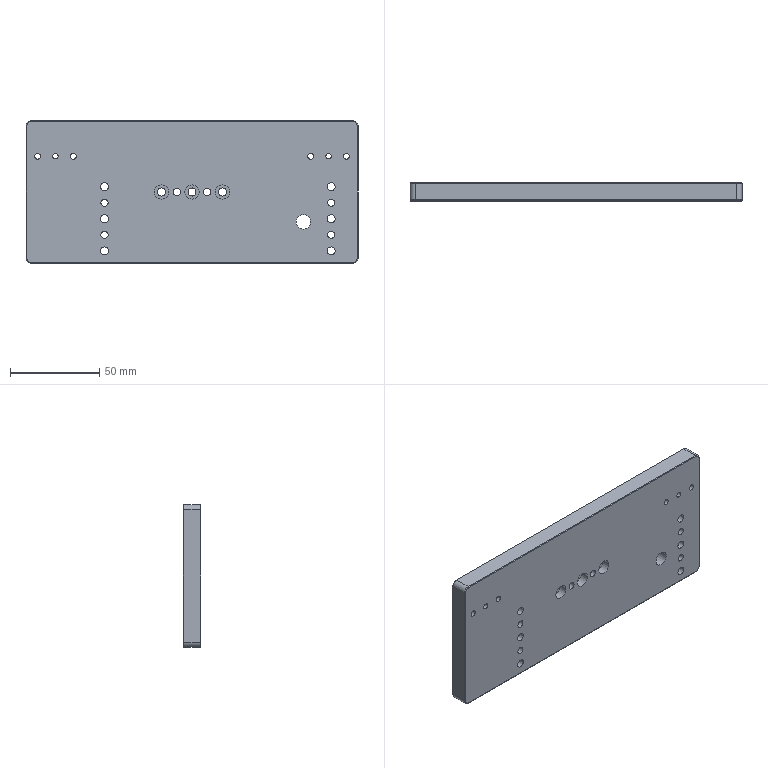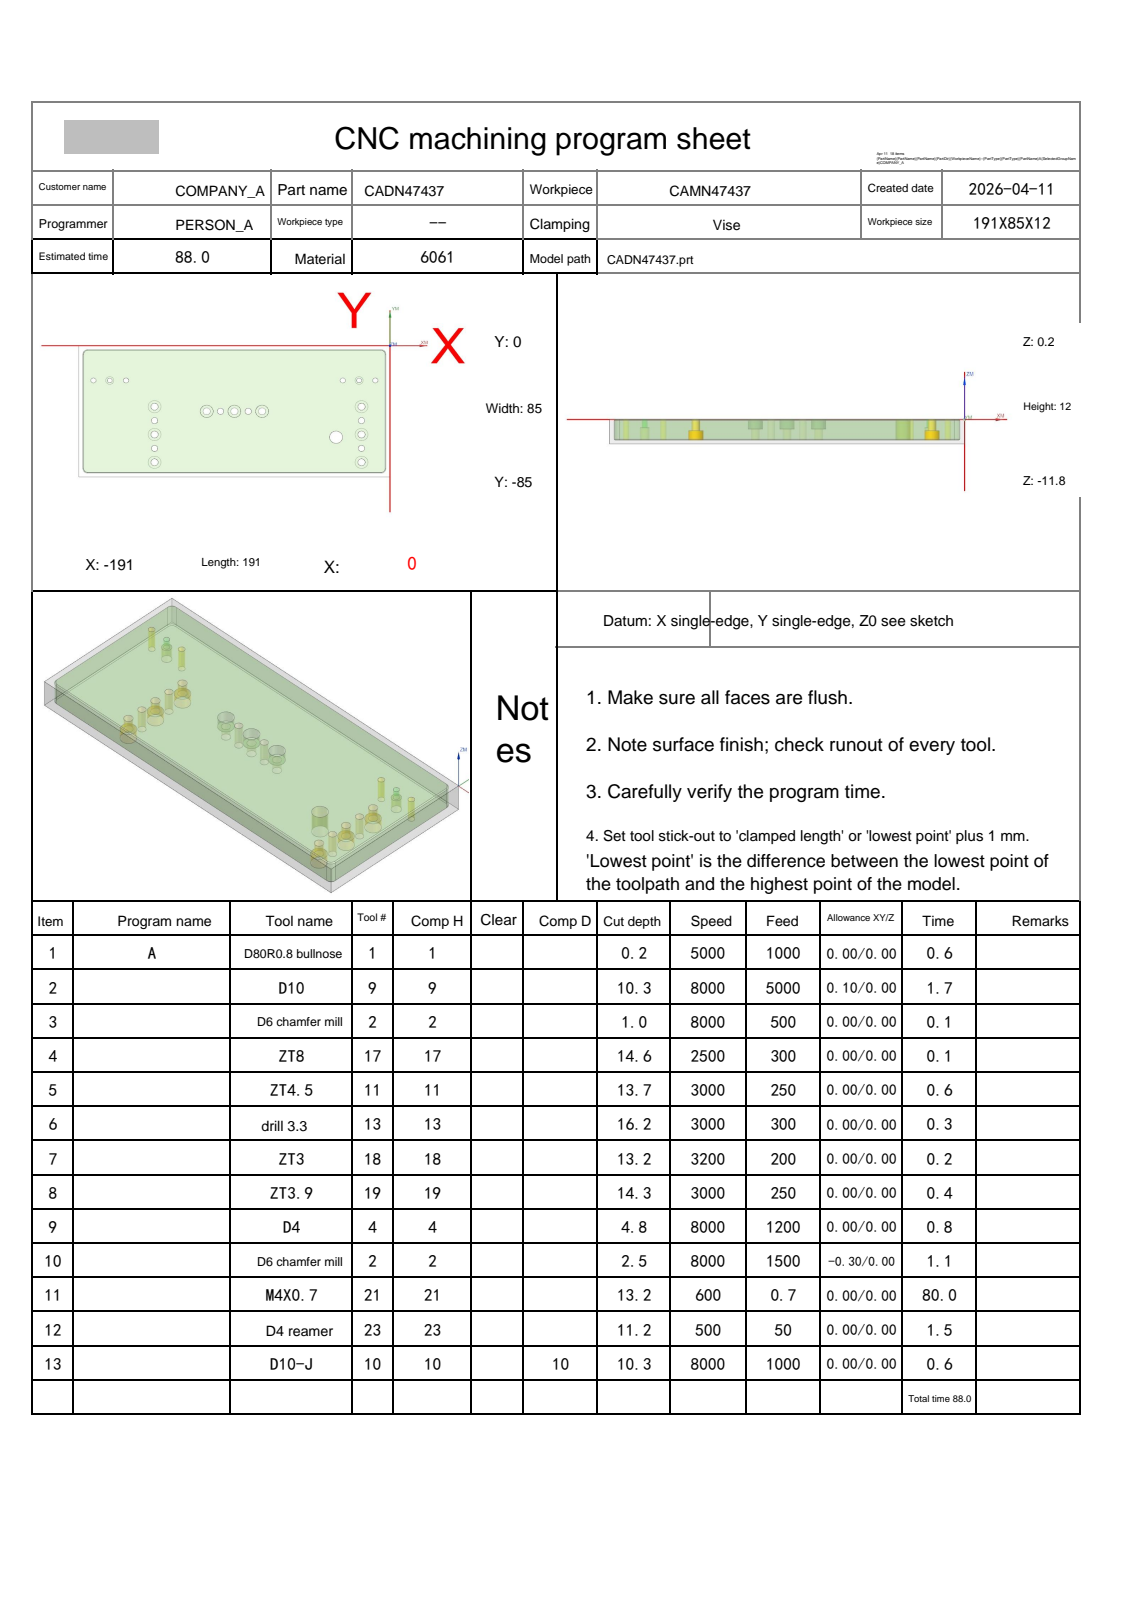NC program | NX | posted by the shop | part box 186 x 10 x 80 mm
Whole program:
%
O0001
(Machine time: 164.60 MIN)
(===Total Tool:12===)
(T1=D80R0.8 bullnose D=80.  R=0.8  D-  H01 Z=-0.   )
(T9=D10     D=10.  R=0.   D-  H09 Z=-10.1 )
(T2=D6 chamfer mill   D=6.   R=0.   D-  H02 Z=-2.3  )
(T17=ZT8    D=8.   DR_a=118 D-  H17 Z=-14.4 )
(T11=ZT4.5  D=4.5  DR_a=118 D-  H11 Z=-13.5 )
(T13=drill 3.3  D=3.3  DR_a=118 D-  H13 Z=-15.99)
(T18=ZT3    D=3.   DR_a=118 D-  H18 Z=-13.  )
(T19=ZT3.9  D=3.9  DR_a=120 D-  H19 Z=-14.13)
(T4=D4      D=4.   R=0.   D4  H04 Z=-4.6  )
(T21=M4X0.7 D=3.3  DR_a=180 D-  H21 Z=-13.  )
(T23=D4 reamer   D=4.   DR_a=180 D-  H23 Z=-11.  )
(T10=D10-J  D=10.  R=0.   D10 H10 Z=-10.1 )
G80 G90 G17 G49 G40
G91 G28 Z0
M01
N1 T01 M06
(D80R0.8 bullnose  D=80. R=0.8 H=01 ce=0.00 di=0.00)
G00 G90 G54 X42.5 Y-69.167 M03 S5000
G43 H01 Z20.
M08
Z2.
G01 Z0.0 F1000.
X37.5
X-228.5
Y-15.833
X37.5
X42.5
Z2.
G00 Z20.
G91 G28 Z0.0
M05
M09
G91 G28 Z0.0
M01
N2 T09 M06
(D10  D=10. R=0. H=09 ce=0.10 di=0.00)
G00 G90 G54 X-95.5 Y2.6 M03 S8000
G43 H09 Z20.
M08
Z.5
G01 X-5.5 Z.378 F5000.
G02 X2.6 Y-5.5 Z.361 I0.0 J-8.1
G01 Y-79.5 Z.261
G02 X-5.5 Y-87.6 Z.243 I-8.1 J0.0
G01 X-185.5 Z0.0
G02 X-193.6 Y-79.5 Z-.018 I0.0 J8.1
G01 Y-5.5 Z-.118
G02 X-185.5 Y2.6 Z-.135 I8.1 J0.0
G01 X-5.5 Z-.379
G02 X2.6 Y-5.5 Z-.396 I0.0 J-8.1
G01 Y-79.5 Z-.497
G02 X-5.5 Y-87.6 Z-.514 I-8.1 J0.0
G01 X-185.5 Z-.758
G02 X-193.6 Y-79.5 Z-.775 I0.0 J8.1
G01 Y-5.5 Z-.875
G02 X-185.5 Y2.6 Z-.892 I8.1 J0.0
G01 X-5.5 Z-1.136
G02 X2.6 Y-5.5 Z-1.153 I0.0 J-8.1
G01 Y-79.5 Z-1.254
G02 X-5.5 Y-87.6 Z-1.271 I-8.1 J0.0
G01 X-185.5 Z-1.515
G02 X-193.6 Y-79.5 Z-1.532 I0.0 J8.1
G01 Y-5.5 Z-1.632
G02 X-185.5 Y2.6 Z-1.65 I8.1 J0.0
G01 X-5.5 Z-1.893
G02 X2.6 Y-5.5 Z-1.911 I0.0 J-8.1
G01 Y-79.5 Z-2.011
G02 X-5.5 Y-87.6 Z-2.028 I-8.1 J0.0
G01 X-185.5 Z-2.272
G02 X-193.6 Y-79.5 Z-2.289 I0.0 J8.1
G01 Y-5.5 Z-2.389
G02 X-185.5 Y2.6 Z-2.407 I8.1 J0.0
G01 X-5.5 Z-2.65
G02 X2.6 Y-5.5 Z-2.668 I0.0 J-8.1
G01 Y-79.5 Z-2.768
G02 X-5.5 Y-87.6 Z-2.785 I-8.1 J0.0
G01 X-185.5 Z-3.029
G02 X-193.6 Y-79.5 Z-3.046 I0.0 J8.1
G01 Y-5.5 Z-3.147
G02 X-185.5 Y2.6 Z-3.164 I8.1 J0.0
G01 X-5.5 Z-3.408
G02 X2.6 Y-5.5 Z-3.425 I0.0 J-8.1
G01 Y-79.5 Z-3.525
G02 X-5.5 Y-87.6 Z-3.542 I-8.1 J0.0
G01 X-185.5 Z-3.786
G02 X-193.6 Y-79.5 Z-3.803 I0.0 J8.1
G01 Y-5.5 Z-3.904
G02 X-185.5 Y2.6 Z-3.921 I8.1 J0.0
G01 X-5.5 Z-4.165
G02 X2.6 Y-5.5 Z-4.182 I0.0 J-8.1
G01 Y-79.5 Z-4.282
G02 X-5.5 Y-87.6 Z-4.3 I-8.1 J0.0
G01 X-185.5 Z-4.543
G02 X-193.6 Y-79.5 Z-4.561 I0.0 J8.1
G01 Y-5.5 Z-4.661
G02 X-185.5 Y2.6 Z-4.678 I8.1 J0.0
G01 X-5.5 Z-4.922
G02 X2.6 Y-5.5 Z-4.939 I0.0 J-8.1
G01 Y-79.5 Z-5.039
G02 X-5.5 Y-87.6 Z-5.057 I-8.1 J0.0
G01 X-185.5 Z-5.3
G02 X-193.6 Y-79.5 Z-5.318 I0.0 J8.1
G01 Y-5.5 Z-5.418
G02 X-185.5 Y2.6 Z-5.435 I8.1 J0.0
G01 X-5.5 Z-5.679
G02 X2.6 Y-5.5 Z-5.696 I0.0 J-8.1
G01 Y-79.5 Z-5.797
G02 X-5.5 Y-87.6 Z-5.814 I-8.1 J0.0
G01 X-185.5 Z-6.058
G02 X-193.6 Y-79.5 Z-6.075 I0.0 J8.1
G01 Y-5.5 Z-6.175
G02 X-185.5 Y2.6 Z-6.192 I8.1 J0.0
G01 X-5.5 Z-6.436
G02 X2.6 Y-5.5 Z-6.453 I0.0 J-8.1
G01 Y-79.5 Z-6.554
G02 X-5.5 Y-87.6 Z-6.571 I-8.1 J0.0
G01 X-185.5 Z-6.815
G02 X-193.6 Y-79.5 Z-6.832 I0.0 J8.1
G01 Y-5.5 Z-6.932
G02 X-185.5 Y2.6 Z-6.95 I8.1 J0.0
G01 X-5.5 Z-7.193
G02 X2.6 Y-5.5 Z-7.211 I0.0 J-8.1
G01 Y-79.5 Z-7.311
G02 X-5.5 Y-87.6 Z-7.328 I-8.1 J0.0
G01 X-185.5 Z-7.572
G02 X-193.6 Y-79.5 Z-7.589 I0.0 J8.1
G01 Y-5.5 Z-7.689
G02 X-185.5 Y2.6 Z-7.707 I8.1 J0.0
G01 X-5.5 Z-7.95
G02 X2.6 Y-5.5 Z-7.968 I0.0 J-8.1
G01 Y-79.5 Z-8.068
G02 X-5.5 Y-87.6 Z-8.085 I-8.1 J0.0
G01 X-185.5 Z-8.329
G02 X-193.6 Y-79.5 Z-8.346 I0.0 J8.1
G01 Y-5.5 Z-8.447
G02 X-185.5 Y2.6 Z-8.464 I8.1 J0.0
G01 X-5.5 Z-8.708
G02 X2.6 Y-5.5 Z-8.725 I0.0 J-8.1
G01 Y-79.5 Z-8.825
G02 X-5.5 Y-87.6 Z-8.842 I-8.1 J0.0
G01 X-185.5 Z-9.086
G02 X-193.6 Y-79.5 Z-9.103 I0.0 J8.1
G01 Y-5.5 Z-9.204
G02 X-185.5 Y2.6 Z-9.221 I8.1 J0.0
G01 X-5.5 Z-9.465
G02 X2.6 Y-5.5 Z-9.482 I0.0 J-8.1
G01 Y-79.5 Z-9.582
G02 X-5.5 Y-87.6 Z-9.6 I-8.1 J0.0
G01 X-185.5 Z-9.843
G02 X-193.6 Y-79.5 Z-9.861 I0.0 J8.1
G01 Y-5.5 Z-9.961
G02 X-185.5 Y2.6 Z-9.978 I8.1 J0.0
G01 X-95.5 Z-10.1
X-5.5
G02 X2.6 Y-5.5 I0.0 J-8.1
G01 Y-79.5
G02 X-5.5 Y-87.6 I-8.1 J0.0
G01 X-185.5
G02 X-193.6 Y-79.5 I0.0 J8.1
G01 Y-5.5
G02 X-185.5 Y2.6 I8.1 J0.0
G01 X-95.5
X-95.
Z-9.1
G00 Z20.
G91 G28 Z0.0
M05
M09
G91 G28 Z0.0
M01
N3 T02 M06
(D6 chamfer mill  D=6. R=0. H=02 ce=0.00 di=0.00)
G00 G90 G54 X-182. Y-22.5 M03 S8000
G43 H02 Z20.
M08
G98 G81 X-182. Y-22.5 Z-.8 R1. F500.
X-172.
X-162.
X-144.5 Y-39.5
Y-48.5
Y-57.5
Y-66.5
Y-75.5
X-112.5 Y-42.5
X-104.
X-95.5
X-87.
X-78.5
X-33.099 Y-59.25
X-17.5 Y-75.5
Y-66.5
Y-57.5
Y-48.5
Y-39.5
X-9. Y-22.5
X-19.
X-29.
G80
G00 Z20.
G91 G28 Z0.0
M05
M09
G91 G28 Z0.0
M01
N4 T17 M06
(ZT8 D=8. DR_a=118 H=17)
G00 G90 G54 X-33.099 Y-59.25 M03 S2500
G43 H17 Z20.
M08
G98 G83 X-33.099 Y-59.25 Z-14.403 R1. F300. Q3.
G80
G00 Z20.
G91 G28 Z0.0
M05
M09
G91 G28 Z0.0
M01
N5 T11 M06
(ZT4.5 D=4.5 DR_a=118 H=11)
G00 G90 G54 X-17.5 Y-75.5 M03 S3000
G43 H11 Z20.
M08
G98 G83 X-17.5 Y-75.5 Z-13.5 R1. F250. Q3.
Y-57.5
Y-39.5
X-144.5
Y-57.5
Y-75.5
G80
G00 Z20.
G00 G90 X-112.5 Y-42.5 M03 S2800
Z20.
G98 G83 X-112.5 Y-42.5 Z-13.352 R1. F200. Q2.
X-95.5
X-78.5
G80
G00 Z20.
G91 G28 Z0.0
M05
M09
G91 G28 Z0.0
M01
N6 T13 M06
(drill 3.3 D=3.3 DR_a=118 H=13)
G00 G90 G54 X-182. Y-22.5 M03 S3000
G43 H13 Z20.
M08
G98 G83 X-182. Y-22.5 Z-15.991 R1. F300. Q2.
X-162.
X-29.
X-9.
G80
G00 Z20.
G91 G28 Z0.0
M05
M09
G91 G28 Z0.0
M01
N7 T18 M06
(ZT3 D=3. DR_a=118 H=18)
G00 G90 G54 X-19. Y-22.5 M03 S3200
G43 H18 Z20.
M08
G98 G83 X-19. Y-22.5 Z-13. R1. F200. Q2.
X-172.
G80
G00 Z20.
G91 G28 Z0.0
M05
M09
G91 G28 Z0.0
M01
N8 T19 M06
(ZT3.9 D=3.9 DR_a=120 H=19)
G00 G90 G54 X-17.5 Y-66.5 M03 S3000
G43 H19 Z20.
M08
G98 G83 X-17.5 Y-66.5 Z-14.126 R1. F250. Q2.
Y-48.5
X-87. Y-42.5
X-104.
X-144.5 Y-48.5
Y-66.5
G80
G00 Z20.
G91 G28 Z0.0
M05
M09
G91 G28 Z0.0
M01
N9 T04 M06
(D4  D=4. R=0. H=04 ce=0.10 di=0.00)
G00 G90 G54 X-112.5 Y-42.5 M03 S8000
G43 H04 Z20.
M08
Z.5
G03 X-111.55 Y-43.45 I.95 J0.0 F1200.
X-110.6 Y-42.5 I0.0 J.95
X-110.6 Y-42.5 Z.2 I-1.9 J0.0
X-110.6 Y-42.5 Z-.1 I-1.9 J0.0
X-110.6 Y-42.5 Z-.4 I-1.9 J0.0
X-110.6 Y-42.5 Z-.7 I-1.9 J0.0
X-110.6 Y-42.5 Z-1. I-1.9 J0.0
X-110.6 Y-42.5 Z-1.3 I-1.9 J0.0
X-110.6 Y-42.5 Z-1.6 I-1.9 J0.0
X-110.6 Y-42.5 Z-1.9 I-1.9 J0.0
X-110.6 Y-42.5 Z-2.2 I-1.9 J0.0
X-110.6 Y-42.5 Z-2.5 I-1.9 J0.0
X-110.6 Y-42.5 Z-2.8 I-1.9 J0.0
X-110.6 Y-42.5 Z-3.1 I-1.9 J0.0
X-110.6 Y-42.5 Z-3.4 I-1.9 J0.0
X-110.6 Y-42.5 Z-3.7 I-1.9 J0.0
X-110.6 Y-42.5 Z-4. I-1.9 J0.0
X-110.6 Y-42.5 Z-4.3 I-1.9 J0.0
X-110.6 Y-42.5 Z-4.6 I-1.9 J0.0
X-112.5 Y-40.6 I-1.9 J0.0
X-114.4 Y-42.5 I0.0 J-1.9
X-112.5 Y-44.4 I1.9 J0.0
X-110.6 Y-42.5 I0.0 J1.9
X-111.55 Y-41.55 I-.95 J0.0
X-112.5 Y-42.5 I0.0 J-.95
G00 Z20.
X-95.5
Z.5
G03 X-94.55 Y-43.45 I.95 J0.0
X-93.6 Y-42.5 I0.0 J.95
X-93.6 Y-42.5 Z.2 I-1.9 J0.0
X-93.6 Y-42.5 Z-.1 I-1.9 J0.0
X-93.6 Y-42.5 Z-.4 I-1.9 J0.0
X-93.6 Y-42.5 Z-.7 I-1.9 J0.0
X-93.6 Y-42.5 Z-1. I-1.9 J0.0
X-93.6 Y-42.5 Z-1.3 I-1.9 J0.0
X-93.6 Y-42.5 Z-1.6 I-1.9 J0.0
X-93.6 Y-42.5 Z-1.9 I-1.9 J0.0
X-93.6 Y-42.5 Z-2.2 I-1.9 J0.0
X-93.6 Y-42.5 Z-2.5 I-1.9 J0.0
X-93.6 Y-42.5 Z-2.8 I-1.9 J0.0
X-93.6 Y-42.5 Z-3.1 I-1.9 J0.0
X-93.6 Y-42.5 Z-3.4 I-1.9 J0.0
X-93.6 Y-42.5 Z-3.7 I-1.9 J0.0
X-93.6 Y-42.5 Z-4. I-1.9 J0.0
X-93.6 Y-42.5 Z-4.3 I-1.9 J0.0
X-93.6 Y-42.5 Z-4.6 I-1.9 J0.0
X-95.5 Y-40.6 I-1.9 J0.0
X-97.4 Y-42.5 I0.0 J-1.9
X-95.5 Y-44.4 I1.9 J0.0
X-93.6 Y-42.5 I0.0 J1.9
X-94.55 Y-41.55 I-.95 J0.0
X-95.5 Y-42.5 I0.0 J-.95
G00 Z20.
X-78.5
Z.5
G03 X-77.55 Y-43.45 I.95 J0.0
X-76.6 Y-42.5 I0.0 J.95
X-76.6 Y-42.5 Z.2 I-1.9 J0.0
X-76.6 Y-42.5 Z-.1 I-1.9 J0.0
X-76.6 Y-42.5 Z-.4 I-1.9 J0.0
X-76.6 Y-42.5 Z-.7 I-1.9 J0.0
X-76.6 Y-42.5 Z-1. I-1.9 J0.0
X-76.6 Y-42.5 Z-1.3 I-1.9 J0.0
X-76.6 Y-42.5 Z-1.6 I-1.9 J0.0
X-76.6 Y-42.5 Z-1.9 I-1.9 J0.0
X-76.6 Y-42.5 Z-2.2 I-1.9 J0.0
X-76.6 Y-42.5 Z-2.5 I-1.9 J0.0
X-76.6 Y-42.5 Z-2.8 I-1.9 J0.0
X-76.6 Y-42.5 Z-3.1 I-1.9 J0.0
X-76.6 Y-42.5 Z-3.4 I-1.9 J0.0
X-76.6 Y-42.5 Z-3.7 I-1.9 J0.0
X-76.6 Y-42.5 Z-4. I-1.9 J0.0
X-76.6 Y-42.5 Z-4.3 I-1.9 J0.0
X-76.6 Y-42.5 Z-4.6 I-1.9 J0.0
X-78.5 Y-40.6 I-1.9 J0.0
X-80.4 Y-42.5 I0.0 J-1.9
X-78.5 Y-44.4 I1.9 J0.0
X-76.6 Y-42.5 I0.0 J1.9
X-77.55 Y-41.55 I-.95 J0.0
X-78.5 Y-42.5 I0.0 J-.95
G00 Z20.
G00 G90 X-112.5 Y-42.5 M03 S8000
Z20.
Z.5
G41 D04
G01 X-112.46 Y-42.696 F500.
G03 X-111.49 Y-43.49 I.97 J.196
X-110.5 Y-42.5 I0.0 J.99
X-110.5 Y-42.5 Z-4.5 I-2. J0.0
X-110.516 Y-42.249 Z-4.6 I-2. J0.0
X-112.5 Y-40.5 I-1.984 J-.251
X-114.5 Y-42.5 I0.0 J-2.
X-112.5 Y-44.5 I2. J0.0
X-110.5 Y-42.5 I0.0 J2.
X-110.516 Y-42.249 I-2. J0.0
X-111.498 Y-41.383 I-.982 J-.124
X-112.485 Y-42.301 I0.0 J-.99
G01 G40 X-112.5 Y-42.5
G00 Z20.
X-95.5
Z.5
G41 D04
G01 X-95.46 Y-42.696
G03 X-94.49 Y-43.49 I.97 J.196
X-93.5 Y-42.5 I0.0 J.99
X-93.5 Y-42.5 Z-4.5 I-2. J0.0
X-93.516 Y-42.249 Z-4.6 I-2. J0.0
X-95.5 Y-40.5 I-1.984 J-.251
X-97.5 Y-42.5 I0.0 J-2.
X-95.5 Y-44.5 I2. J0.0
X-93.5 Y-42.5 I0.0 J2.
X-93.516 Y-42.249 I-2. J0.0
X-94.498 Y-41.383 I-.982 J-.124
X-95.485 Y-42.301 I0.0 J-.99
G01 G40 X-95.5 Y-42.5
G00 Z20.
X-78.5
Z.5
G41 D04
G01 X-78.46 Y-42.696
G03 X-77.49 Y-43.49 I.97 J.196
X-76.5 Y-42.5 I0.0 J.99
X-76.5 Y-42.5 Z-4.5 I-2. J0.0
X-76.516 Y-42.249 Z-4.6 I-2. J0.0
X-78.5 Y-40.5 I-1.984 J-.251
X-80.5 Y-42.5 I0.0 J-2.
X-78.5 Y-44.5 I2. J0.0
X-76.5 Y-42.5 I0.0 J2.
X-76.516 Y-42.249 I-2. J0.0
X-77.498 Y-41.383 I-.982 J-.124
X-78.485 Y-42.301 I0.0 J-.99
G01 G40 X-78.5 Y-42.5
G00 Z20.
G91 G28 Z0.0
M05
M09
G91 G28 Z0.0
M01
N10 T02 M06
(D6 chamfer mill  D=6. R=0. H=02 ce=0.00 di=0.00)
G00 G90 G54 X-19. Y-22.5 M03 S8000
G43 H02 Z20.
M08
G98 G81 X-19. Y-22.5 Z-1.8 R3. F500.
X-172.
G80
G00 Z20.
G00 G90 X-182. Y-22.5 M03 S8000
Z20.
G98 G81 X-182. Y-22.5 Z-2.2 R3. F500.
X-162.
X-29.
X-9.
G80
G00 Z20.
G00 G90 X-17.5 Y-66.5 M03 S8000
Z20.
G98 G81 X-17.5 Y-66.5 Z-2.3 R3. F500.
Y-48.5
X-87. Y-42.5
X-104.
X-144.5 Y-48.5
Y-66.5
G80
G00 Z20.
G00 G90 X-143.95 Y-75.482 M03 S8000
Z20.
Z-.5
G01 Z-1. F500.
X-143. Y-75.45
G03 X-144.5 Y-73.95 I-1.5 J0.0
X-146.05 Y-75.5 I0.0 J-1.55
X-144.5 Y-77.05 I1.55 J0.0
X-142.95 Y-75.5 I0.0 J1.55
X-144.5 Y-73.95 I-1.55 J0.0
X-146. Y-75.45 I0.0 J-1.5
G01 X-145.05 Y-75.482
Z-.5
G00 Z20.
X-143.95 Y-57.482
Z-.5
G01 Z-1.
X-143. Y-57.45
G03 X-144.5 Y-55.95 I-1.5 J0.0
X-146.05 Y-57.5 I0.0 J-1.55
X-144.5 Y-59.05 I1.55 J0.0
X-142.95 Y-57.5 I0.0 J1.55
X-144.5 Y-55.95 I-1.55 J0.0
X-146. Y-57.45 I0.0 J-1.5
G01 X-145.05 Y-57.482
Z-.5
G00 Z20.
X-143.95 Y-39.482
Z-.5
G01 Z-1.
X-143. Y-39.45
G03 X-144.5 Y-37.95 I-1.5 J0.0
X-146.05 Y-39.5 I0.0 J-1.55
X-144.5 Y-41.05 I1.55 J0.0
X-142.95 Y-39.5 I0.0 J1.55
X-144.5 Y-37.95 I-1.55 J0.0
X-146. Y-39.45 I0.0 J-1.5
G01 X-145.05 Y-39.482
Z-.5
G00 Z20.
X-16.95
Z-.5
G01 Z-1.
X-16. Y-39.45
G03 X-17.5 Y-37.95 I-1.5 J0.0
X-19.05 Y-39.5 I0.0 J-1.55
X-17.5 Y-41.05 I1.55 J0.0
X-15.95 Y-39.5 I0.0 J1.55
X-17.5 Y-37.95 I-1.55 J0.0
X-19. Y-39.45 I0.0 J-1.5
G01 X-18.05 Y-39.482
Z-.5
G00 Z20.
X-16.95 Y-57.482
Z-.5
G01 Z-1.
X-16. Y-57.45
G03 X-17.5 Y-55.95 I-1.5 J0.0
X-19.05 Y-57.5 I0.0 J-1.55
X-17.5 Y-59.05 I1.55 J0.0
X-15.95 Y-57.5 I0.0 J1.55
X-17.5 Y-55.95 I-1.55 J0.0
X-19. Y-57.45 I0.0 J-1.5
G01 X-18.05 Y-57.482
Z-.5
G00 Z20.
X-16.95 Y-75.482
Z-.5
G01 Z-1.
X-16. Y-75.45
G03 X-17.5 Y-73.95 I-1.5 J0.0
X-19.05 Y-75.5 I0.0 J-1.55
X-17.5 Y-77.05 I1.55 J0.0
X-15.95 Y-75.5 I0.0 J1.55
X-17.5 Y-73.95 I-1.55 J0.0
X-19. Y-75.45 I0.0 J-1.5
G01 X-18.05 Y-75.482
Z-.5
G00 Z20.
G00 G90 X-111.753 Y-45.712 M03 S8000
Z20.
Z2.5
G01 X-111.538 Y-45.66 Z2.42 F500.
X-111.172 Y-45.524 Z2.278
X-110.825 Y-45.347 Z2.136
X-110.501 Y-45.129 Z1.994
X-110.205 Y-44.875 Z1.852
X-109.941 Y-44.588 Z1.71
X-109.712 Y-44.272 Z1.568
X-109.572 Y-44.028 Z1.465
X-109.412 Y-43.672 Z1.323
X-109.295 Y-43.3 Z1.181
X-109.223 Y-42.916 Z1.039
X-109.197 Y-42.527 Z.897
X-109.217 Y-42.138 Z.755
X-109.283 Y-41.753 Z.613
X-109.393 Y-41.379 Z.471
X-109.547 Y-41.02 Z.329
X-109.742 Y-40.682 Z.187
X-109.976 Y-40.37 Z.045
X-110.244 Y-40.087 Z-.097
X-110.545 Y-39.838 Z-.239
X-110.872 Y-39.626 Z-.381
X-111.222 Y-39.454 Z-.523
X-111.59 Y-39.325 Z-.665
X-111.971 Y-39.24 Z-.807
X-112.359 Y-39.2 Z-.949
X-112.5 Z-1.
G03 X-115.8 Y-42.5 I0.0 J-3.3
X-112.5 Y-45.8 I3.3 J0.0
X-109.2 Y-42.5 I0.0 J3.3
X-112.5 Y-39.2 I-3.3 J0.0
X-112.998 Y-39.238 I0.0 J-3.3
G01 Z1.5
G00 Z20.
X-94.753 Y-45.712
Z2.5
G01 X-94.538 Y-45.66 Z2.42
X-94.172 Y-45.524 Z2.278
X-93.825 Y-45.347 Z2.136
X-93.501 Y-45.129 Z1.994
X-93.205 Y-44.875 Z1.852
X-92.941 Y-44.588 Z1.71
X-92.712 Y-44.272 Z1.568
X-92.572 Y-44.028 Z1.465
X-92.412 Y-43.672 Z1.323
X-92.295 Y-43.3 Z1.181
X-92.223 Y-42.916 Z1.039
X-92.197 Y-42.527 Z.897
X-92.217 Y-42.138 Z.755
X-92.283 Y-41.753 Z.613
X-92.393 Y-41.379 Z.471
X-92.547 Y-41.02 Z.329
X-92.742 Y-40.682 Z.187
X-92.976 Y-40.37 Z.045
X-93.244 Y-40.087 Z-.097
X-93.545 Y-39.838 Z-.239
X-93.872 Y-39.626 Z-.381
X-94.222 Y-39.454 Z-.523
X-94.59 Y-39.325 Z-.665
X-94.971 Y-39.24 Z-.807
X-95.359 Y-39.2 Z-.949
X-95.5 Z-1.
G03 X-98.8 Y-42.5 I0.0 J-3.3
X-95.5 Y-45.8 I3.3 J0.0
X-92.2 Y-42.5 I0.0 J3.3
X-95.5 Y-39.2 I-3.3 J0.0
X-95.998 Y-39.238 I0.0 J-3.3
G01 Z1.5
G00 Z20.
X-77.753 Y-45.712
Z2.5
G01 X-77.538 Y-45.66 Z2.42
X-77.172 Y-45.524 Z2.278
X-76.825 Y-45.347 Z2.136
X-76.501 Y-45.129 Z1.994
X-76.205 Y-44.875 Z1.852
X-75.941 Y-44.588 Z1.71
X-75.712 Y-44.272 Z1.568
X-75.572 Y-44.028 Z1.465
X-75.412 Y-43.672 Z1.323
X-75.295 Y-43.3 Z1.181
X-75.223 Y-42.916 Z1.039
X-75.197 Y-42.527 Z.897
X-75.217 Y-42.138 Z.755
X-75.283 Y-41.753 Z.613
X-75.393 Y-41.379 Z.471
X-75.547 Y-41.02 Z.329
X-75.742 Y-40.682 Z.187
X-75.976 Y-40.37 Z.045
X-76.244 Y-40.087 Z-.097
X-76.545 Y-39.838 Z-.239
X-76.872 Y-39.626 Z-.381
X-77.222 Y-39.454 Z-.523
X-77.59 Y-39.325 Z-.665
X-77.971 Y-39.24 Z-.807
X-78.359 Y-39.2 Z-.949
X-78.5 Z-1.
G03 X-81.8 Y-42.5 I0.0 J-3.3
X-78.5 Y-45.8 I3.3 J0.0
X-75.2 Y-42.5 I0.0 J3.3
X-78.5 Y-39.2 I-3.3 J0.0
X-78.998 Y-39.238 I0.0 J-3.3
G01 Z1.5
G00 Z20.
G00 G90 X-30.81 Y-59.021 M03 S8000
Z20.
Z-.5
G01 Z-1. F800.
X-30.099 Y-58.95
G03 X-33.099 Y-55.95 I-3. J0.0
X-36.399 Y-59.25 I0.0 J-3.3
X-33.099 Y-62.55 I3.3 J0.0
X-29.799 Y-59.25 I0.0 J3.3
X-33.099 Y-55.95 I-3.3 J0.0
X-36.099 Y-58.95 I0.0 J-3.
G01 X-35.388 Y-59.021
Z-.5
G00 Z20.
G00 G90 X-4.309 Y-84.253 M03 S6500
Z20.
Z.3
G01 Z-1.2 F1500.
G03 X-5.5 Y-83.2 I-1.191 J-.147
G01 X-185.5
G02 X-186.225 Y-83.128 I0.0 J3.7
G01 X-186.274 Y-83.118
G02 X-189.2 Y-79.5 I.774 J3.618
G01 Y-5.5
G02 X-188.166 Y-2.935 I3.7 J0.0
X-188.006 Y-2.778 I2.666 J-2.565
X-187.335 Y-2.287 I2.506 J-2.722
G01 X-187.265 Y-2.248
G02 X-185.5 Y-1.8 I1.765 J-3.252
G01 X-5.5
G02 X-1.8 Y-5.5 I0.0 J-3.7
G01 Y-79.5
G02 X-5.5 Y-83.2 I-3.7 J0.0
G01 X-5.9
G03 X-7.1 Y-84.4 I0.0 J-1.2
G01 Z.3
G00 Z20.
G91 G28 Z0.0
M05
M09
G91 G28 Z0.0
M01
N11 T21 M06
(M4X0.7 D=3.3 DR_a=180 H=21)
G00 G90 G54 X-182. Y-22.5 M03 S600
G43 H21 Z20.
M08
G95
G98 G84 X-182. Y-22.5 Z-13. R1. F.7 Q4.
X-162.
X-29.
X-9.
G80
G94
G00 Z20.
G91 G28 Z0.0
M05
M09
G91 G28 Z0.0
M01
N12 T23 M06
(D4 reamer D=4. DR_a=180 H=23)
G00 G90 G54 X-17.5 Y-66.5 M03 S500
G43 H23 Z20.
M08
G98 G81 X-17.5 Y-66.5 Z-11. R1. F50.
Y-48.5
X-87. Y-42.5
X-104.
X-144.5 Y-48.5
Y-66.5
G80
G00 Z20.
G91 G28 Z0.0
M05
M09
G91 G28 Z0.0
M01
N13 T10 M06
(D10-J  D=10. R=0. H=10 ce=0.00 di=0.00)
G00 G90 G54 X-186.51 Y3.644 M03 S8000
G43 H10 Z20.
M08
Z-9.6
G01 Z-10.1 F1000.
G41 D10
X-186.498 Y3.444
G03 X-185.5 Y2.5 I.998 J.056
G01 X-5.5
G02 X2.5 Y-5.5 I0.0 J-8.
G01 Y-79.5
G02 X-5.5 Y-87.5 I-8. J0.0
G01 X-185.5
G02 X-193.5 Y-79.5 I0.0 J8.
G01 Y-5.5
G02 X-185.5 Y2.5 I8. J0.0
G01 X-185.
G03 X-184. Y3.5 I0.0 J1.
G01 G40 Y3.7
Z-9.6
G00 Z20.
M05
M09
G91 G28 Z0.0
G91 G28 Y0.0
M30
%